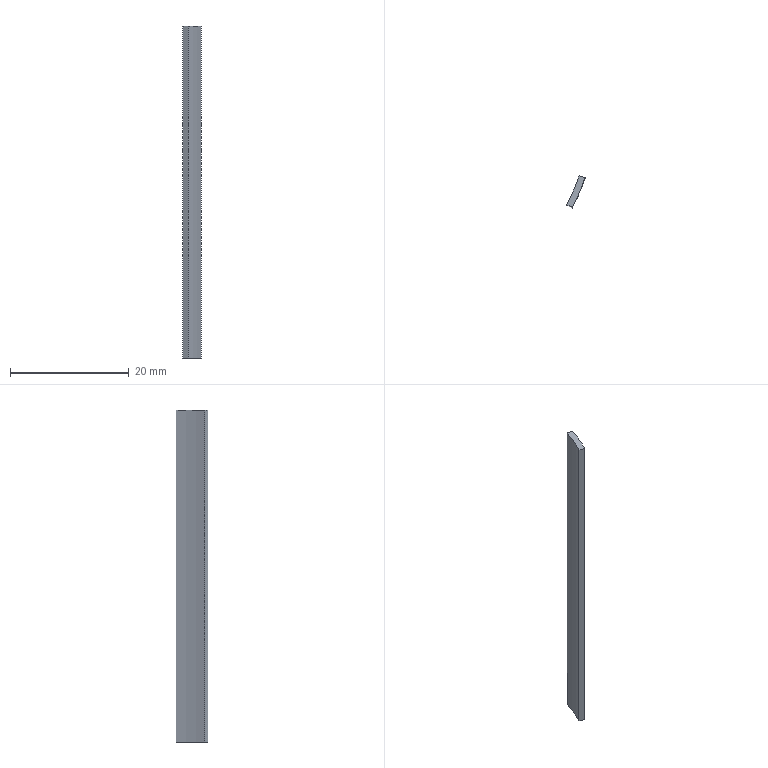Part | NX | features BREP 2 | 2 solids | 12 faces | box 3.074 x 5.341 x 56 mm | volume 634.023 mm3 | plane 8 | cylinder 4 | commonest cylinder face diameters 69.173 x2 72.496 x2
STEP:
#1=CARTESIAN_POINT('',(-0.6018,-2.695,-4.));
#2=VERTEX_POINT('',#1);
#3=CARTESIAN_POINT('',(-0.6018,-2.695,52.));
#4=VERTEX_POINT('',#3);
#5=CARTESIAN_POINT('',(-0.6018,-2.695,0.));
#6=DIRECTION('',(0.,0.,1.));
#7=VECTOR('',#6,1000.);
#8=LINE('',#5,#7);
#9=EDGE_CURVE('',#2,#4,#8,.T.);
#10=ORIENTED_EDGE('',*,*,#9,.T.);
#11=CARTESIAN_POINT('',(-1.512,-2.217,52.));
#12=VERTEX_POINT('',#11);
#13=CARTESIAN_POINT('',(-17.052,5.948,52.));
#14=DIRECTION('',(0.8853,-0.4651,0.));
#15=VECTOR('',#14,1000.);
#16=LINE('',#13,#15);
#17=EDGE_CURVE('',#12,#4,#16,.T.);
#18=ORIENTED_EDGE('',*,*,#17,.F.);
#19=CARTESIAN_POINT('',(-1.512,-2.217,-4.));
#20=VERTEX_POINT('',#19);
#21=CARTESIAN_POINT('',(-1.512,-2.217,0.));
#22=DIRECTION('',(0.,0.,1.));
#23=VECTOR('',#22,1000.);
#24=LINE('',#21,#23);
#25=EDGE_CURVE('',#20,#12,#24,.T.);
#26=ORIENTED_EDGE('',*,*,#25,.F.);
#27=CARTESIAN_POINT('',(-17.052,5.948,-4.));
#28=DIRECTION('',(0.8853,-0.4651,0.));
#29=VECTOR('',#28,1000.);
#30=LINE('',#27,#29);
#31=EDGE_CURVE('',#20,#2,#30,.T.);
#32=ORIENTED_EDGE('',*,*,#31,.T.);
#33=EDGE_LOOP('',(#10,#18,#26,#32));
#34=FACE_BOUND('',#33,.T.);
#35=CARTESIAN_POINT('',(-17.052,5.948,0.));
#36=DIRECTION('',(-0.4651,-0.8853,0.));
#37=DIRECTION('',(-0.8853,0.4651,0.));
#38=AXIS2_PLACEMENT_3D('',#35,#36,#37);
#39=PLANE('',#38);
#40=ADVANCED_FACE('',(#34),#39,.T.);
#41=ORIENTED_EDGE('',*,*,#25,.T.);
#42=CARTESIAN_POINT('',(0.5334,2.645,52.));
#43=VERTEX_POINT('',#42);
#44=CARTESIAN_POINT('',(-32.277,13.585,52.));
#45=DIRECTION('',(0.,0.,-1.));
#46=DIRECTION('',(1.,0.,0.));
#47=AXIS2_PLACEMENT_3D('',#44,#45,#46);
#48=CIRCLE('',#47,34.586);
#49=EDGE_CURVE('',#43,#12,#48,.T.);
#50=ORIENTED_EDGE('',*,*,#49,.F.);
#51=CARTESIAN_POINT('',(0.5334,2.645,-4.));
#52=VERTEX_POINT('',#51);
#53=CARTESIAN_POINT('',(0.5334,2.645,0.));
#54=DIRECTION('',(0.,0.,1.));
#55=VECTOR('',#54,1000.);
#56=LINE('',#53,#55);
#57=EDGE_CURVE('',#52,#43,#56,.T.);
#58=ORIENTED_EDGE('',*,*,#57,.F.);
#59=CARTESIAN_POINT('',(-32.277,13.585,-4.));
#60=DIRECTION('',(0.,0.,-1.));
#61=DIRECTION('',(1.,0.,0.));
#62=AXIS2_PLACEMENT_3D('',#59,#60,#61);
#63=CIRCLE('',#62,34.586);
#64=EDGE_CURVE('',#52,#20,#63,.T.);
#65=ORIENTED_EDGE('',*,*,#64,.T.);
#66=EDGE_LOOP('',(#41,#50,#58,#65));
#67=FACE_BOUND('',#66,.T.);
#68=CARTESIAN_POINT('',(-32.277,13.585,0.));
#69=DIRECTION('',(0.,0.,1.));
#70=DIRECTION('',(-1.,0.,0.));
#71=AXIS2_PLACEMENT_3D('',#68,#69,#70);
#72=CYLINDRICAL_SURFACE('',#71,34.586);
#73=ADVANCED_FACE('',(#67),#72,.F.);
#74=ORIENTED_EDGE('',*,*,#57,.T.);
#75=CARTESIAN_POINT('',(1.562,2.302,52.));
#76=VERTEX_POINT('',#75);
#77=CARTESIAN_POINT('',(-13.76,7.411,52.));
#78=DIRECTION('',(-0.9487,0.3163,0.));
#79=VECTOR('',#78,1000.);
#80=LINE('',#77,#79);
#81=EDGE_CURVE('',#76,#43,#80,.T.);
#82=ORIENTED_EDGE('',*,*,#81,.F.);
#83=CARTESIAN_POINT('',(1.562,2.302,-4.));
#84=VERTEX_POINT('',#83);
#85=CARTESIAN_POINT('',(1.562,2.302,0.));
#86=DIRECTION('',(0.,0.,1.));
#87=VECTOR('',#86,1000.);
#88=LINE('',#85,#87);
#89=EDGE_CURVE('',#84,#76,#88,.T.);
#90=ORIENTED_EDGE('',*,*,#89,.F.);
#91=CARTESIAN_POINT('',(-13.76,7.411,-4.));
#92=DIRECTION('',(-0.9487,0.3163,0.));
#93=VECTOR('',#92,1000.);
#94=LINE('',#91,#93);
#95=EDGE_CURVE('',#84,#52,#94,.T.);
#96=ORIENTED_EDGE('',*,*,#95,.T.);
#97=EDGE_LOOP('',(#74,#82,#90,#96));
#98=FACE_BOUND('',#97,.T.);
#99=CARTESIAN_POINT('',(-13.76,7.411,0.));
#100=DIRECTION('',(-0.3163,-0.9487,0.));
#101=DIRECTION('',(-0.9487,0.3163,0.));
#102=AXIS2_PLACEMENT_3D('',#99,#100,#101);
#103=PLANE('',#102);
#104=ADVANCED_FACE('',(#98),#103,.F.);
#105=CARTESIAN_POINT('',(-32.69,14.164,-4.));
#106=DIRECTION('',(0.,0.,1.));
#107=DIRECTION('',(1.,0.,0.));
#108=AXIS2_PLACEMENT_3D('',#105,#106,#107);
#109=CIRCLE('',#108,36.248);
#110=EDGE_CURVE('',#2,#84,#109,.T.);
#111=ORIENTED_EDGE('',*,*,#110,.T.);
#112=ORIENTED_EDGE('',*,*,#89,.T.);
#113=CARTESIAN_POINT('',(-32.69,14.164,52.));
#114=DIRECTION('',(0.,0.,1.));
#115=DIRECTION('',(1.,0.,0.));
#116=AXIS2_PLACEMENT_3D('',#113,#114,#115);
#117=CIRCLE('',#116,36.248);
#118=EDGE_CURVE('',#4,#76,#117,.T.);
#119=ORIENTED_EDGE('',*,*,#118,.F.);
#120=ORIENTED_EDGE('',*,*,#9,.F.);
#121=EDGE_LOOP('',(#111,#112,#119,#120));
#122=FACE_BOUND('',#121,.T.);
#123=CARTESIAN_POINT('',(-32.69,14.164,0.));
#124=DIRECTION('',(0.,0.,1.));
#125=DIRECTION('',(-1.,0.,0.));
#126=AXIS2_PLACEMENT_3D('',#123,#124,#125);
#127=CYLINDRICAL_SURFACE('',#126,36.248);
#128=ADVANCED_FACE('',(#122),#127,.T.);
#129=ORIENTED_EDGE('',*,*,#81,.T.);
#130=ORIENTED_EDGE('',*,*,#49,.T.);
#131=ORIENTED_EDGE('',*,*,#17,.T.);
#132=ORIENTED_EDGE('',*,*,#118,.T.);
#133=EDGE_LOOP('',(#129,#130,#131,#132));
#134=FACE_BOUND('',#133,.T.);
#135=CARTESIAN_POINT('',(-9.377,20.555,52.));
#136=DIRECTION('',(0.,0.,1.));
#137=DIRECTION('',(-1.,0.,0.));
#138=AXIS2_PLACEMENT_3D('',#135,#136,#137);
#139=PLANE('',#138);
#140=ADVANCED_FACE('',(#134),#139,.T.);
#141=ORIENTED_EDGE('',*,*,#95,.F.);
#142=ORIENTED_EDGE('',*,*,#110,.F.);
#143=ORIENTED_EDGE('',*,*,#31,.F.);
#144=ORIENTED_EDGE('',*,*,#64,.F.);
#145=EDGE_LOOP('',(#141,#142,#143,#144));
#146=FACE_BOUND('',#145,.T.);
#147=CARTESIAN_POINT('',(-9.377,20.555,-4.));
#148=DIRECTION('',(0.,0.,1.));
#149=DIRECTION('',(-1.,0.,0.));
#150=AXIS2_PLACEMENT_3D('',#147,#148,#149);
#151=PLANE('',#150);
#152=ADVANCED_FACE('',(#146),#151,.F.);
#153=CLOSED_SHELL('',(#40,#73,#104,#128,#140,#152));
#154=MANIFOLD_SOLID_BREP('',#153);
#155=CARTESIAN_POINT('',(-0.6018,-2.695,-4.));
#156=VERTEX_POINT('',#155);
#157=CARTESIAN_POINT('',(-0.6018,-2.695,52.));
#158=VERTEX_POINT('',#157);
#159=CARTESIAN_POINT('',(-0.6018,-2.695,0.));
#160=DIRECTION('',(0.,0.,1.));
#161=VECTOR('',#160,1000.);
#162=LINE('',#159,#161);
#163=EDGE_CURVE('',#156,#158,#162,.T.);
#164=ORIENTED_EDGE('',*,*,#163,.T.);
#165=CARTESIAN_POINT('',(-1.512,-2.217,52.));
#166=VERTEX_POINT('',#165);
#167=CARTESIAN_POINT('',(-17.052,5.948,52.));
#168=DIRECTION('',(0.8853,-0.4651,0.));
#169=VECTOR('',#168,1000.);
#170=LINE('',#167,#169);
#171=EDGE_CURVE('',#166,#158,#170,.T.);
#172=ORIENTED_EDGE('',*,*,#171,.F.);
#173=CARTESIAN_POINT('',(-1.512,-2.217,-4.));
#174=VERTEX_POINT('',#173);
#175=CARTESIAN_POINT('',(-1.512,-2.217,0.));
#176=DIRECTION('',(0.,0.,1.));
#177=VECTOR('',#176,1000.);
#178=LINE('',#175,#177);
#179=EDGE_CURVE('',#174,#166,#178,.T.);
#180=ORIENTED_EDGE('',*,*,#179,.F.);
#181=CARTESIAN_POINT('',(-17.052,5.948,-4.));
#182=DIRECTION('',(0.8853,-0.4651,0.));
#183=VECTOR('',#182,1000.);
#184=LINE('',#181,#183);
#185=EDGE_CURVE('',#174,#156,#184,.T.);
#186=ORIENTED_EDGE('',*,*,#185,.T.);
#187=EDGE_LOOP('',(#164,#172,#180,#186));
#188=FACE_BOUND('',#187,.T.);
#189=CARTESIAN_POINT('',(-17.052,5.948,0.));
#190=DIRECTION('',(-0.4651,-0.8853,0.));
#191=DIRECTION('',(-0.8853,0.4651,0.));
#192=AXIS2_PLACEMENT_3D('',#189,#190,#191);
#193=PLANE('',#192);
#194=ADVANCED_FACE('',(#188),#193,.T.);
#195=ORIENTED_EDGE('',*,*,#179,.T.);
#196=CARTESIAN_POINT('',(0.5334,2.645,52.));
#197=VERTEX_POINT('',#196);
#198=CARTESIAN_POINT('',(-32.277,13.585,52.));
#199=DIRECTION('',(0.,0.,-1.));
#200=DIRECTION('',(1.,0.,0.));
#201=AXIS2_PLACEMENT_3D('',#198,#199,#200);
#202=CIRCLE('',#201,34.586);
#203=EDGE_CURVE('',#197,#166,#202,.T.);
#204=ORIENTED_EDGE('',*,*,#203,.F.);
#205=CARTESIAN_POINT('',(0.5334,2.645,-4.));
#206=VERTEX_POINT('',#205);
#207=CARTESIAN_POINT('',(0.5334,2.645,0.));
#208=DIRECTION('',(0.,0.,1.));
#209=VECTOR('',#208,1000.);
#210=LINE('',#207,#209);
#211=EDGE_CURVE('',#206,#197,#210,.T.);
#212=ORIENTED_EDGE('',*,*,#211,.F.);
#213=CARTESIAN_POINT('',(-32.277,13.585,-4.));
#214=DIRECTION('',(0.,0.,-1.));
#215=DIRECTION('',(1.,0.,0.));
#216=AXIS2_PLACEMENT_3D('',#213,#214,#215);
#217=CIRCLE('',#216,34.586);
#218=EDGE_CURVE('',#206,#174,#217,.T.);
#219=ORIENTED_EDGE('',*,*,#218,.T.);
#220=EDGE_LOOP('',(#195,#204,#212,#219));
#221=FACE_BOUND('',#220,.T.);
#222=CARTESIAN_POINT('',(-32.277,13.585,0.));
#223=DIRECTION('',(0.,0.,1.));
#224=DIRECTION('',(-1.,0.,0.));
#225=AXIS2_PLACEMENT_3D('',#222,#223,#224);
#226=CYLINDRICAL_SURFACE('',#225,34.586);
#227=ADVANCED_FACE('',(#221),#226,.F.);
#228=ORIENTED_EDGE('',*,*,#211,.T.);
#229=CARTESIAN_POINT('',(1.562,2.302,52.));
#230=VERTEX_POINT('',#229);
#231=CARTESIAN_POINT('',(-13.76,7.411,52.));
#232=DIRECTION('',(-0.9487,0.3163,0.));
#233=VECTOR('',#232,1000.);
#234=LINE('',#231,#233);
#235=EDGE_CURVE('',#230,#197,#234,.T.);
#236=ORIENTED_EDGE('',*,*,#235,.F.);
#237=CARTESIAN_POINT('',(1.562,2.302,-4.));
#238=VERTEX_POINT('',#237);
#239=CARTESIAN_POINT('',(1.562,2.302,0.));
#240=DIRECTION('',(0.,0.,1.));
#241=VECTOR('',#240,1000.);
#242=LINE('',#239,#241);
#243=EDGE_CURVE('',#238,#230,#242,.T.);
#244=ORIENTED_EDGE('',*,*,#243,.F.);
#245=CARTESIAN_POINT('',(-13.76,7.411,-4.));
#246=DIRECTION('',(-0.9487,0.3163,0.));
#247=VECTOR('',#246,1000.);
#248=LINE('',#245,#247);
#249=EDGE_CURVE('',#238,#206,#248,.T.);
#250=ORIENTED_EDGE('',*,*,#249,.T.);
#251=EDGE_LOOP('',(#228,#236,#244,#250));
#252=FACE_BOUND('',#251,.T.);
#253=CARTESIAN_POINT('',(-13.76,7.411,0.));
#254=DIRECTION('',(-0.3163,-0.9487,0.));
#255=DIRECTION('',(-0.9487,0.3163,0.));
#256=AXIS2_PLACEMENT_3D('',#253,#254,#255);
#257=PLANE('',#256);
#258=ADVANCED_FACE('',(#252),#257,.F.);
#259=CARTESIAN_POINT('',(-32.69,14.164,-4.));
#260=DIRECTION('',(0.,0.,1.));
#261=DIRECTION('',(1.,0.,0.));
#262=AXIS2_PLACEMENT_3D('',#259,#260,#261);
#263=CIRCLE('',#262,36.248);
#264=EDGE_CURVE('',#156,#238,#263,.T.);
#265=ORIENTED_EDGE('',*,*,#264,.T.);
#266=ORIENTED_EDGE('',*,*,#243,.T.);
#267=CARTESIAN_POINT('',(-32.69,14.164,52.));
#268=DIRECTION('',(0.,0.,1.));
#269=DIRECTION('',(1.,0.,0.));
#270=AXIS2_PLACEMENT_3D('',#267,#268,#269);
#271=CIRCLE('',#270,36.248);
#272=EDGE_CURVE('',#158,#230,#271,.T.);
#273=ORIENTED_EDGE('',*,*,#272,.F.);
#274=ORIENTED_EDGE('',*,*,#163,.F.);
#275=EDGE_LOOP('',(#265,#266,#273,#274));
#276=FACE_BOUND('',#275,.T.);
#277=CARTESIAN_POINT('',(-32.69,14.164,0.));
#278=DIRECTION('',(0.,0.,1.));
#279=DIRECTION('',(-1.,0.,0.));
#280=AXIS2_PLACEMENT_3D('',#277,#278,#279);
#281=CYLINDRICAL_SURFACE('',#280,36.248);
#282=ADVANCED_FACE('',(#276),#281,.T.);
#283=ORIENTED_EDGE('',*,*,#235,.T.);
#284=ORIENTED_EDGE('',*,*,#203,.T.);
#285=ORIENTED_EDGE('',*,*,#171,.T.);
#286=ORIENTED_EDGE('',*,*,#272,.T.);
#287=EDGE_LOOP('',(#283,#284,#285,#286));
#288=FACE_BOUND('',#287,.T.);
#289=CARTESIAN_POINT('',(-9.377,20.555,52.));
#290=DIRECTION('',(0.,0.,1.));
#291=DIRECTION('',(-1.,0.,0.));
#292=AXIS2_PLACEMENT_3D('',#289,#290,#291);
#293=PLANE('',#292);
#294=ADVANCED_FACE('',(#288),#293,.T.);
#295=ORIENTED_EDGE('',*,*,#249,.F.);
#296=ORIENTED_EDGE('',*,*,#264,.F.);
#297=ORIENTED_EDGE('',*,*,#185,.F.);
#298=ORIENTED_EDGE('',*,*,#218,.F.);
#299=EDGE_LOOP('',(#295,#296,#297,#298));
#300=FACE_BOUND('',#299,.T.);
#301=CARTESIAN_POINT('',(-9.377,20.555,-4.));
#302=DIRECTION('',(0.,0.,1.));
#303=DIRECTION('',(-1.,0.,0.));
#304=AXIS2_PLACEMENT_3D('',#301,#302,#303);
#305=PLANE('',#304);
#306=ADVANCED_FACE('',(#300),#305,.F.);
#307=CLOSED_SHELL('',(#194,#227,#258,#282,#294,#306));
#308=MANIFOLD_SOLID_BREP('',#307);
#309=(LENGTH_UNIT()NAMED_UNIT(*)SI_UNIT(.MILLI.,.METRE.));
#310=UNCERTAINTY_MEASURE_WITH_UNIT(LENGTH_MEASURE(0.00001),#309,'','');
#311=(NAMED_UNIT(*)PLANE_ANGLE_UNIT()SI_UNIT($,.RADIAN.));
#312=(NAMED_UNIT(*)SI_UNIT($,.STERADIAN.)SOLID_ANGLE_UNIT());
#313=(GEOMETRIC_REPRESENTATION_CONTEXT(3)GLOBAL_UNCERTAINTY_ASSIGNED_CONTEXT((#310))GLOBAL_UNIT_ASSIGNED_CONTEXT((#309,#311,#312))REPRESENTATION_CONTEXT('',''));
#314=ADVANCED_BREP_SHAPE_REPRESENTATION('',(#154,#308),#313);